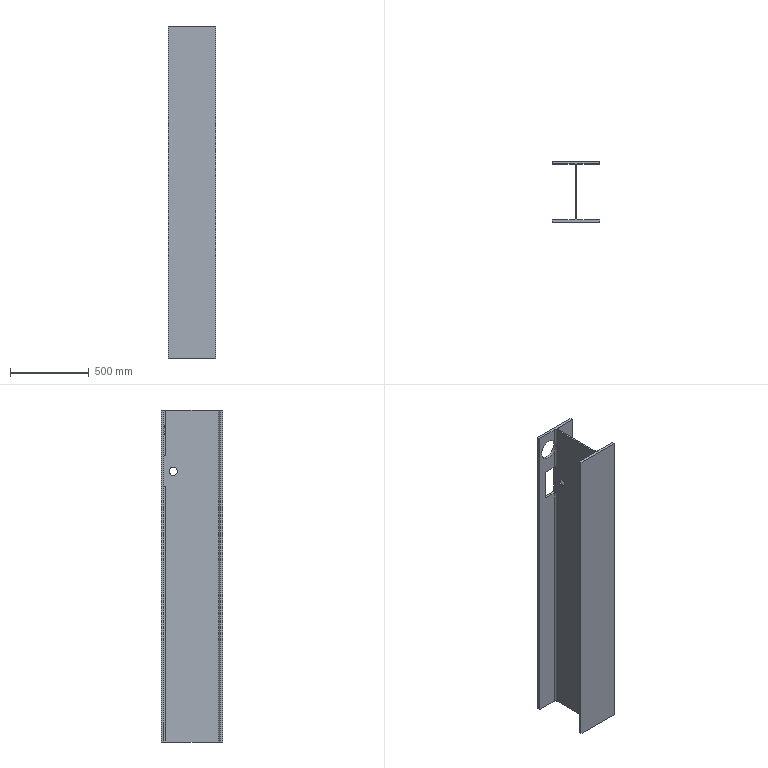Part | SolidWorks | features ICE 2, Extrusion 1 | 1 solid | 26 faces | box 300 x 390 x 2113 mm | volume 27642804 mm3 | plane 17 | cylinder 9 | commonest cylinder face diameters 26 x5 51 x2 125 x2
STEP:
#1=CARTESIAN_POINT('',(155.,289.5,1723.));
#2=VERTEX_POINT('',#1);
#3=CARTESIAN_POINT('',(155.,340.5,1723.));
#4=VERTEX_POINT('',#3);
#5=CARTESIAN_POINT('',(155.,315.,1723.));
#6=DIRECTION('',(1.,0.,0.));
#7=DIRECTION('',(0.,0.,1.));
#8=AXIS2_PLACEMENT_3D('',#5,#6,#7);
#9=CIRCLE('',#8,25.5);
#10=EDGE_CURVE('',#2,#4,#9,.T.);
#11=ORIENTED_EDGE('',*,*,#10,.T.);
#12=CARTESIAN_POINT('',(145.,340.5,1723.));
#13=VERTEX_POINT('',#12);
#14=CARTESIAN_POINT('',(300.001,340.5,1723.));
#15=DIRECTION('',(-1.,0.,0.));
#16=VECTOR('',#15,1000.);
#17=LINE('',#14,#16);
#18=EDGE_CURVE('',#4,#13,#17,.T.);
#19=ORIENTED_EDGE('',*,*,#18,.T.);
#20=CARTESIAN_POINT('',(145.,289.5,1723.));
#21=VERTEX_POINT('',#20);
#22=CARTESIAN_POINT('',(145.,315.,1723.));
#23=DIRECTION('',(-1.,0.,0.));
#24=DIRECTION('',(0.,-1.,0.));
#25=AXIS2_PLACEMENT_3D('',#22,#23,#24);
#26=CIRCLE('',#25,25.5);
#27=EDGE_CURVE('',#13,#21,#26,.T.);
#28=ORIENTED_EDGE('',*,*,#27,.T.);
#29=CARTESIAN_POINT('',(300.001,289.5,1723.));
#30=DIRECTION('',(-1.,0.,0.));
#31=VECTOR('',#30,1000.);
#32=LINE('',#29,#31);
#33=EDGE_CURVE('',#2,#21,#32,.T.);
#34=ORIENTED_EDGE('',*,*,#33,.F.);
#35=EDGE_LOOP('',(#11,#19,#28,#34));
#36=FACE_OUTER_BOUND('',#35,.T.);
#37=CARTESIAN_POINT('',(300.001,315.,1723.));
#38=DIRECTION('',(-1.,0.,0.));
#39=DIRECTION('',(0.,-1.,0.));
#40=AXIS2_PLACEMENT_3D('',#37,#38,#39);
#41=CYLINDRICAL_SURFACE('',#40,25.5);
#42=ADVANCED_FACE('',(#36),#41,.F.);
#43=CARTESIAN_POINT('',(82.,374.,2048.5));
#44=VERTEX_POINT('',#43);
#45=CARTESIAN_POINT('',(82.,374.,1923.5));
#46=VERTEX_POINT('',#45);
#47=CARTESIAN_POINT('',(82.,374.,1986.));
#48=DIRECTION('',(0.,-1.,0.));
#49=DIRECTION('',(-1.,0.,0.));
#50=AXIS2_PLACEMENT_3D('',#47,#48,#49);
#51=CIRCLE('',#50,62.5);
#52=EDGE_CURVE('',#44,#46,#51,.T.);
#53=ORIENTED_EDGE('',*,*,#52,.T.);
#54=CARTESIAN_POINT('',(82.,390.,1923.5));
#55=VERTEX_POINT('',#54);
#56=CARTESIAN_POINT('',(82.,-0.001,1923.5));
#57=DIRECTION('',(0.,1.,0.));
#58=VECTOR('',#57,1000.);
#59=LINE('',#56,#58);
#60=EDGE_CURVE('',#46,#55,#59,.T.);
#61=ORIENTED_EDGE('',*,*,#60,.T.);
#62=CARTESIAN_POINT('',(82.,390.,2048.5));
#63=VERTEX_POINT('',#62);
#64=CARTESIAN_POINT('',(82.,390.,1986.));
#65=DIRECTION('',(0.,1.,0.));
#66=DIRECTION('',(0.,0.,1.));
#67=AXIS2_PLACEMENT_3D('',#64,#65,#66);
#68=CIRCLE('',#67,62.5);
#69=EDGE_CURVE('',#55,#63,#68,.T.);
#70=ORIENTED_EDGE('',*,*,#69,.T.);
#71=CARTESIAN_POINT('',(82.,-0.001,2048.5));
#72=DIRECTION('',(0.,1.,0.));
#73=VECTOR('',#72,1000.);
#74=LINE('',#71,#73);
#75=EDGE_CURVE('',#44,#63,#74,.T.);
#76=ORIENTED_EDGE('',*,*,#75,.F.);
#77=EDGE_LOOP('',(#53,#61,#70,#76));
#78=FACE_OUTER_BOUND('',#77,.T.);
#79=CARTESIAN_POINT('',(82.,-0.001,1986.));
#80=DIRECTION('',(0.,1.,0.));
#81=DIRECTION('',(0.,0.,1.));
#82=AXIS2_PLACEMENT_3D('',#79,#80,#81);
#83=CYLINDRICAL_SURFACE('',#82,62.5);
#84=ADVANCED_FACE('',(#78),#83,.F.);
#85=CARTESIAN_POINT('',(132.,374.,1948.5));
#86=VERTEX_POINT('',#85);
#87=CARTESIAN_POINT('',(132.,374.,1823.));
#88=VERTEX_POINT('',#87);
#89=CARTESIAN_POINT('',(132.,374.,2113.));
#90=DIRECTION('',(0.,0.,-1.));
#91=VECTOR('',#90,1000.);
#92=LINE('',#89,#91);
#93=EDGE_CURVE('',#86,#88,#92,.T.);
#94=ORIENTED_EDGE('',*,*,#93,.T.);
#95=CARTESIAN_POINT('',(145.,361.,1823.));
#96=VERTEX_POINT('',#95);
#97=CARTESIAN_POINT('',(132.,361.,1823.));
#98=DIRECTION('',(0.,0.,1.));
#99=DIRECTION('',(1.,0.,0.));
#100=AXIS2_PLACEMENT_3D('',#97,#98,#99);
#101=CIRCLE('',#100,13.);
#102=EDGE_CURVE('',#96,#88,#101,.T.);
#103=ORIENTED_EDGE('',*,*,#102,.F.);
#104=CARTESIAN_POINT('',(145.,361.,2113.));
#105=VERTEX_POINT('',#104);
#106=CARTESIAN_POINT('',(145.,361.,2113.));
#107=DIRECTION('',(0.,0.,-1.));
#108=VECTOR('',#107,1000.);
#109=LINE('',#106,#108);
#110=EDGE_CURVE('',#105,#96,#109,.T.);
#111=ORIENTED_EDGE('',*,*,#110,.F.);
#112=CARTESIAN_POINT('',(132.,374.,2113.));
#113=VERTEX_POINT('',#112);
#114=CARTESIAN_POINT('',(132.,361.,2113.));
#115=DIRECTION('',(0.,0.,-1.));
#116=DIRECTION('',(-1.,0.,0.));
#117=AXIS2_PLACEMENT_3D('',#114,#115,#116);
#118=CIRCLE('',#117,13.);
#119=EDGE_CURVE('',#113,#105,#118,.T.);
#120=ORIENTED_EDGE('',*,*,#119,.F.);
#121=CARTESIAN_POINT('',(132.,374.,2023.5));
#122=VERTEX_POINT('',#121);
#123=CARTESIAN_POINT('',(132.,374.,2113.));
#124=DIRECTION('',(0.,0.,-1.));
#125=VECTOR('',#124,1000.);
#126=LINE('',#123,#125);
#127=EDGE_CURVE('',#113,#122,#126,.T.);
#128=ORIENTED_EDGE('',*,*,#127,.T.);
#129=CARTESIAN_POINT('',(132.,374.,1948.5));
#130=CARTESIAN_POINT('',(133.05,374.,1949.9));
#131=CARTESIAN_POINT('',(134.027,373.875,1951.324));
#132=CARTESIAN_POINT('',(135.848,373.452,1954.227));
#133=CARTESIAN_POINT('',(136.693,373.154,1955.705));
#134=CARTESIAN_POINT('',(137.866,372.609,1957.964));
#135=CARTESIAN_POINT('',(138.242,372.411,1958.726));
#136=CARTESIAN_POINT('',(138.957,371.99,1960.254));
#137=CARTESIAN_POINT('',(139.297,371.767,1961.019));
#138=CARTESIAN_POINT('',(140.264,371.067,1963.32));
#139=CARTESIAN_POINT('',(140.84,370.561,1964.862));
#140=CARTESIAN_POINT('',(141.865,369.499,1967.968));
#141=CARTESIAN_POINT('',(142.313,368.944,1969.532));
#142=CARTESIAN_POINT('',(143.089,367.82,1972.693));
#143=CARTESIAN_POINT('',(143.415,367.25,1974.289));
#144=CARTESIAN_POINT('',(143.813,366.435,1976.725));
#145=CARTESIAN_POINT('',(143.931,366.169,1977.545));
#146=CARTESIAN_POINT('',(144.134,365.673,1979.194));
#147=CARTESIAN_POINT('',(144.219,365.443,1980.023));
#148=CARTESIAN_POINT('',(144.357,365.043,1981.694));
#149=CARTESIAN_POINT('',(144.41,364.875,1982.537));
#150=CARTESIAN_POINT('',(144.481,364.638,1984.243));
#151=CARTESIAN_POINT('',(144.5,364.571,1985.107));
#152=CARTESIAN_POINT('',(144.5,364.57,1986.424));
#153=CARTESIAN_POINT('',(144.496,364.586,1986.863));
#154=CARTESIAN_POINT('',(144.478,364.649,1987.731));
#155=CARTESIAN_POINT('',(144.464,364.695,1988.161));
#156=CARTESIAN_POINT('',(144.411,364.871,1989.444));
#157=CARTESIAN_POINT('',(144.358,365.039,1990.288));
#158=CARTESIAN_POINT('',(144.221,365.438,1991.961));
#159=CARTESIAN_POINT('',(144.136,365.669,1992.79));
#160=CARTESIAN_POINT('',(143.933,366.164,1994.438));
#161=CARTESIAN_POINT('',(143.816,366.429,1995.259));
#162=CARTESIAN_POINT('',(143.418,367.245,1997.698));
#163=CARTESIAN_POINT('',(143.091,367.816,1999.298));
#164=CARTESIAN_POINT('',(142.314,368.943,2002.465));
#165=CARTESIAN_POINT('',(141.864,369.5,2004.033));
#166=CARTESIAN_POINT('',(140.836,370.564,2007.148));
#167=CARTESIAN_POINT('',(140.258,371.072,2008.695));
#168=CARTESIAN_POINT('',(139.286,371.774,2011.004));
#169=CARTESIAN_POINT('',(138.944,371.998,2011.775));
#170=CARTESIAN_POINT('',(138.228,372.418,2013.301));
#171=CARTESIAN_POINT('',(137.855,372.615,2014.057));
#172=CARTESIAN_POINT('',(136.686,373.156,2016.307));
#173=CARTESIAN_POINT('',(135.844,373.454,2017.78));
#174=CARTESIAN_POINT('',(134.026,373.875,2020.676));
#175=CARTESIAN_POINT('',(133.05,374.,2022.099));
#176=CARTESIAN_POINT('',(132.,374.,2023.5));
#177=B_SPLINE_CURVE_WITH_KNOTS('',3,(#129,#130,#131,#132,#133,#134,#135,#136,#137,#138,#139,#140,#141,#142,#143,#144,#145,#146,#147,#148,#149,#150,#151,#152,#153,#154,#155,#156,#157,#158,#159,#160,#161,#162,#163,#164,#165,#166,#167,#168,#169,#170,#171,#172,#173,#174,#175,#176),.UNSPECIFIED.,.F.,.F.,(4,2,2,2,2,2,2,2,2,2,2,2,2,2,2,2,2,2,2,2,2,2,2,4),(0.,0.005179,0.01036,0.01295,0.01554,0.02071,0.02589,0.03107,0.03366,0.03625,0.03884,0.04143,0.04272,0.04402,0.04661,0.0492,0.05179,0.05696,0.06214,0.06732,0.06991,0.0725,0.07768,0.08286),.UNSPECIFIED.);
#178=EDGE_CURVE('',#86,#122,#177,.T.);
#179=ORIENTED_EDGE('',*,*,#178,.F.);
#180=EDGE_LOOP('',(#94,#103,#111,#120,#128,#179));
#181=FACE_OUTER_BOUND('',#180,.T.);
#182=CARTESIAN_POINT('',(132.,361.,2113.));
#183=DIRECTION('',(0.,0.,-1.));
#184=DIRECTION('',(-1.,0.,0.));
#185=AXIS2_PLACEMENT_3D('',#182,#183,#184);
#186=CYLINDRICAL_SURFACE('',#185,13.);
#187=ADVANCED_FACE('',(#181),#186,.F.);
#188=CARTESIAN_POINT('',(0.,16.,0.));
#189=VERTEX_POINT('',#188);
#190=CARTESIAN_POINT('',(0.,0.,0.));
#191=VERTEX_POINT('',#190);
#192=CARTESIAN_POINT('',(0.,16.,0.));
#193=DIRECTION('',(0.,-1.,0.));
#194=VECTOR('',#193,1000.);
#195=LINE('',#192,#194);
#196=EDGE_CURVE('',#189,#191,#195,.T.);
#197=ORIENTED_EDGE('',*,*,#196,.T.);
#198=CARTESIAN_POINT('',(0.,0.,2113.));
#199=VERTEX_POINT('',#198);
#200=CARTESIAN_POINT('',(0.,0.,2113.));
#201=DIRECTION('',(0.,0.,-1.));
#202=VECTOR('',#201,1000.);
#203=LINE('',#200,#202);
#204=EDGE_CURVE('',#199,#191,#203,.T.);
#205=ORIENTED_EDGE('',*,*,#204,.F.);
#206=CARTESIAN_POINT('',(0.,16.,2113.));
#207=VERTEX_POINT('',#206);
#208=CARTESIAN_POINT('',(0.,16.,2113.));
#209=DIRECTION('',(0.,-1.,0.));
#210=VECTOR('',#209,1000.);
#211=LINE('',#208,#210);
#212=EDGE_CURVE('',#207,#199,#211,.T.);
#213=ORIENTED_EDGE('',*,*,#212,.F.);
#214=CARTESIAN_POINT('',(0.,16.,2113.));
#215=DIRECTION('',(0.,0.,-1.));
#216=VECTOR('',#215,1000.);
#217=LINE('',#214,#216);
#218=EDGE_CURVE('',#207,#189,#217,.T.);
#219=ORIENTED_EDGE('',*,*,#218,.T.);
#220=EDGE_LOOP('',(#197,#205,#213,#219));
#221=FACE_OUTER_BOUND('',#220,.T.);
#222=CARTESIAN_POINT('',(0.,16.,2113.));
#223=DIRECTION('',(1.,0.,0.));
#224=DIRECTION('',(0.,1.,0.));
#225=AXIS2_PLACEMENT_3D('',#222,#223,#224);
#226=PLANE('',#225);
#227=ADVANCED_FACE('',(#221),#226,.F.);
#228=CARTESIAN_POINT('',(300.,0.,0.));
#229=VERTEX_POINT('',#228);
#230=CARTESIAN_POINT('',(0.,0.,0.));
#231=DIRECTION('',(1.,0.,0.));
#232=VECTOR('',#231,1000.);
#233=LINE('',#230,#232);
#234=EDGE_CURVE('',#191,#229,#233,.T.);
#235=ORIENTED_EDGE('',*,*,#234,.T.);
#236=CARTESIAN_POINT('',(300.,0.,2113.));
#237=VERTEX_POINT('',#236);
#238=CARTESIAN_POINT('',(300.,0.,2113.));
#239=DIRECTION('',(0.,0.,-1.));
#240=VECTOR('',#239,1000.);
#241=LINE('',#238,#240);
#242=EDGE_CURVE('',#237,#229,#241,.T.);
#243=ORIENTED_EDGE('',*,*,#242,.F.);
#244=CARTESIAN_POINT('',(0.,0.,2113.));
#245=DIRECTION('',(1.,0.,0.));
#246=VECTOR('',#245,1000.);
#247=LINE('',#244,#246);
#248=EDGE_CURVE('',#199,#237,#247,.T.);
#249=ORIENTED_EDGE('',*,*,#248,.F.);
#250=ORIENTED_EDGE('',*,*,#204,.T.);
#251=EDGE_LOOP('',(#235,#243,#249,#250));
#252=FACE_OUTER_BOUND('',#251,.T.);
#253=CARTESIAN_POINT('',(0.,0.,2113.));
#254=DIRECTION('',(0.,1.,0.));
#255=DIRECTION('',(0.,0.,1.));
#256=AXIS2_PLACEMENT_3D('',#253,#254,#255);
#257=PLANE('',#256);
#258=ADVANCED_FACE('',(#252),#257,.F.);
#259=CARTESIAN_POINT('',(300.,16.,0.));
#260=VERTEX_POINT('',#259);
#261=CARTESIAN_POINT('',(300.,0.,0.));
#262=DIRECTION('',(0.,1.,0.));
#263=VECTOR('',#262,1000.);
#264=LINE('',#261,#263);
#265=EDGE_CURVE('',#229,#260,#264,.T.);
#266=ORIENTED_EDGE('',*,*,#265,.T.);
#267=CARTESIAN_POINT('',(300.,16.,2113.));
#268=VERTEX_POINT('',#267);
#269=CARTESIAN_POINT('',(300.,16.,2113.));
#270=DIRECTION('',(0.,0.,-1.));
#271=VECTOR('',#270,1000.);
#272=LINE('',#269,#271);
#273=EDGE_CURVE('',#268,#260,#272,.T.);
#274=ORIENTED_EDGE('',*,*,#273,.F.);
#275=CARTESIAN_POINT('',(300.,0.,2113.));
#276=DIRECTION('',(0.,1.,0.));
#277=VECTOR('',#276,1000.);
#278=LINE('',#275,#277);
#279=EDGE_CURVE('',#237,#268,#278,.T.);
#280=ORIENTED_EDGE('',*,*,#279,.F.);
#281=ORIENTED_EDGE('',*,*,#242,.T.);
#282=EDGE_LOOP('',(#266,#274,#280,#281));
#283=FACE_OUTER_BOUND('',#282,.T.);
#284=CARTESIAN_POINT('',(300.,0.,2113.));
#285=DIRECTION('',(-1.,0.,0.));
#286=DIRECTION('',(0.,0.,1.));
#287=AXIS2_PLACEMENT_3D('',#284,#285,#286);
#288=PLANE('',#287);
#289=ADVANCED_FACE('',(#283),#288,.F.);
#290=CARTESIAN_POINT('',(168.,16.,0.));
#291=VERTEX_POINT('',#290);
#292=CARTESIAN_POINT('',(300.,16.,0.));
#293=DIRECTION('',(-1.,0.,0.));
#294=VECTOR('',#293,1000.);
#295=LINE('',#292,#294);
#296=EDGE_CURVE('',#260,#291,#295,.T.);
#297=ORIENTED_EDGE('',*,*,#296,.T.);
#298=CARTESIAN_POINT('',(168.,16.,2113.));
#299=VERTEX_POINT('',#298);
#300=CARTESIAN_POINT('',(168.,16.,2113.));
#301=DIRECTION('',(0.,0.,-1.));
#302=VECTOR('',#301,1000.);
#303=LINE('',#300,#302);
#304=EDGE_CURVE('',#299,#291,#303,.T.);
#305=ORIENTED_EDGE('',*,*,#304,.F.);
#306=CARTESIAN_POINT('',(300.,16.,2113.));
#307=DIRECTION('',(-1.,0.,0.));
#308=VECTOR('',#307,1000.);
#309=LINE('',#306,#308);
#310=EDGE_CURVE('',#268,#299,#309,.T.);
#311=ORIENTED_EDGE('',*,*,#310,.F.);
#312=ORIENTED_EDGE('',*,*,#273,.T.);
#313=EDGE_LOOP('',(#297,#305,#311,#312));
#314=FACE_OUTER_BOUND('',#313,.T.);
#315=CARTESIAN_POINT('',(300.,16.,2113.));
#316=DIRECTION('',(0.,-1.,0.));
#317=DIRECTION('',(1.,0.,0.));
#318=AXIS2_PLACEMENT_3D('',#315,#316,#317);
#319=PLANE('',#318);
#320=ADVANCED_FACE('',(#314),#319,.F.);
#321=CARTESIAN_POINT('',(155.,29.,0.));
#322=VERTEX_POINT('',#321);
#323=CARTESIAN_POINT('',(168.,29.,0.));
#324=DIRECTION('',(0.,0.,-1.));
#325=DIRECTION('',(-1.,0.,0.));
#326=AXIS2_PLACEMENT_3D('',#323,#324,#325);
#327=CIRCLE('',#326,13.);
#328=EDGE_CURVE('',#291,#322,#327,.T.);
#329=ORIENTED_EDGE('',*,*,#328,.T.);
#330=CARTESIAN_POINT('',(155.,29.,2113.));
#331=VERTEX_POINT('',#330);
#332=CARTESIAN_POINT('',(155.,29.,2113.));
#333=DIRECTION('',(0.,0.,-1.));
#334=VECTOR('',#333,1000.);
#335=LINE('',#332,#334);
#336=EDGE_CURVE('',#331,#322,#335,.T.);
#337=ORIENTED_EDGE('',*,*,#336,.F.);
#338=CARTESIAN_POINT('',(168.,29.,2113.));
#339=DIRECTION('',(0.,0.,-1.));
#340=DIRECTION('',(-1.,0.,0.));
#341=AXIS2_PLACEMENT_3D('',#338,#339,#340);
#342=CIRCLE('',#341,13.);
#343=EDGE_CURVE('',#299,#331,#342,.T.);
#344=ORIENTED_EDGE('',*,*,#343,.F.);
#345=ORIENTED_EDGE('',*,*,#304,.T.);
#346=EDGE_LOOP('',(#329,#337,#344,#345));
#347=FACE_OUTER_BOUND('',#346,.T.);
#348=CARTESIAN_POINT('',(168.,29.,2113.));
#349=DIRECTION('',(0.,0.,-1.));
#350=DIRECTION('',(-1.,0.,0.));
#351=AXIS2_PLACEMENT_3D('',#348,#349,#350);
#352=CYLINDRICAL_SURFACE('',#351,13.);
#353=ADVANCED_FACE('',(#347),#352,.F.);
#354=ORIENTED_EDGE('',*,*,#10,.F.);
#355=CARTESIAN_POINT('',(155.,315.,1723.));
#356=DIRECTION('',(1.,0.,0.));
#357=DIRECTION('',(0.,0.,1.));
#358=AXIS2_PLACEMENT_3D('',#355,#356,#357);
#359=CIRCLE('',#358,25.5);
#360=EDGE_CURVE('',#4,#2,#359,.T.);
#361=ORIENTED_EDGE('',*,*,#360,.F.);
#362=EDGE_LOOP('',(#354,#361));
#363=FACE_BOUND('',#362,.T.);
#364=CARTESIAN_POINT('',(155.,361.,0.));
#365=VERTEX_POINT('',#364);
#366=CARTESIAN_POINT('',(155.,29.,0.));
#367=DIRECTION('',(0.,1.,0.));
#368=VECTOR('',#367,1000.);
#369=LINE('',#366,#368);
#370=EDGE_CURVE('',#322,#365,#369,.T.);
#371=ORIENTED_EDGE('',*,*,#370,.T.);
#372=CARTESIAN_POINT('',(155.,361.,2113.));
#373=VERTEX_POINT('',#372);
#374=CARTESIAN_POINT('',(155.,361.,2113.));
#375=DIRECTION('',(0.,0.,-1.));
#376=VECTOR('',#375,1000.);
#377=LINE('',#374,#376);
#378=EDGE_CURVE('',#373,#365,#377,.T.);
#379=ORIENTED_EDGE('',*,*,#378,.F.);
#380=CARTESIAN_POINT('',(155.,29.,2113.));
#381=DIRECTION('',(0.,1.,0.));
#382=VECTOR('',#381,1000.);
#383=LINE('',#380,#382);
#384=EDGE_CURVE('',#331,#373,#383,.T.);
#385=ORIENTED_EDGE('',*,*,#384,.F.);
#386=ORIENTED_EDGE('',*,*,#336,.T.);
#387=EDGE_LOOP('',(#371,#379,#385,#386));
#388=FACE_OUTER_BOUND('',#387,.T.);
#389=CARTESIAN_POINT('',(155.,29.,2113.));
#390=DIRECTION('',(-1.,0.,0.));
#391=DIRECTION('',(0.,0.,1.));
#392=AXIS2_PLACEMENT_3D('',#389,#390,#391);
#393=PLANE('',#392);
#394=ADVANCED_FACE('',(#363,#388),#393,.F.);
#395=CARTESIAN_POINT('',(168.,374.,0.));
#396=VERTEX_POINT('',#395);
#397=CARTESIAN_POINT('',(168.,361.,0.));
#398=DIRECTION('',(0.,0.,-1.));
#399=DIRECTION('',(-1.,0.,0.));
#400=AXIS2_PLACEMENT_3D('',#397,#398,#399);
#401=CIRCLE('',#400,13.);
#402=EDGE_CURVE('',#365,#396,#401,.T.);
#403=ORIENTED_EDGE('',*,*,#402,.T.);
#404=CARTESIAN_POINT('',(168.,374.,2113.));
#405=VERTEX_POINT('',#404);
#406=CARTESIAN_POINT('',(168.,374.,2113.));
#407=DIRECTION('',(0.,0.,-1.));
#408=VECTOR('',#407,1000.);
#409=LINE('',#406,#408);
#410=EDGE_CURVE('',#405,#396,#409,.T.);
#411=ORIENTED_EDGE('',*,*,#410,.F.);
#412=CARTESIAN_POINT('',(168.,361.,2113.));
#413=DIRECTION('',(0.,0.,-1.));
#414=DIRECTION('',(-1.,0.,0.));
#415=AXIS2_PLACEMENT_3D('',#412,#413,#414);
#416=CIRCLE('',#415,13.);
#417=EDGE_CURVE('',#373,#405,#416,.T.);
#418=ORIENTED_EDGE('',*,*,#417,.F.);
#419=ORIENTED_EDGE('',*,*,#378,.T.);
#420=EDGE_LOOP('',(#403,#411,#418,#419));
#421=FACE_OUTER_BOUND('',#420,.T.);
#422=CARTESIAN_POINT('',(168.,361.,2113.));
#423=DIRECTION('',(0.,0.,-1.));
#424=DIRECTION('',(-1.,0.,0.));
#425=AXIS2_PLACEMENT_3D('',#422,#423,#424);
#426=CYLINDRICAL_SURFACE('',#425,13.);
#427=ADVANCED_FACE('',(#421),#426,.F.);
#428=CARTESIAN_POINT('',(300.,374.,0.));
#429=VERTEX_POINT('',#428);
#430=CARTESIAN_POINT('',(168.,374.,0.));
#431=DIRECTION('',(1.,0.,0.));
#432=VECTOR('',#431,1000.);
#433=LINE('',#430,#432);
#434=EDGE_CURVE('',#396,#429,#433,.T.);
#435=ORIENTED_EDGE('',*,*,#434,.T.);
#436=CARTESIAN_POINT('',(300.,374.,2113.));
#437=VERTEX_POINT('',#436);
#438=CARTESIAN_POINT('',(300.,374.,2113.));
#439=DIRECTION('',(0.,0.,-1.));
#440=VECTOR('',#439,1000.);
#441=LINE('',#438,#440);
#442=EDGE_CURVE('',#437,#429,#441,.T.);
#443=ORIENTED_EDGE('',*,*,#442,.F.);
#444=CARTESIAN_POINT('',(168.,374.,2113.));
#445=DIRECTION('',(1.,0.,0.));
#446=VECTOR('',#445,1000.);
#447=LINE('',#444,#446);
#448=EDGE_CURVE('',#405,#437,#447,.T.);
#449=ORIENTED_EDGE('',*,*,#448,.F.);
#450=ORIENTED_EDGE('',*,*,#410,.T.);
#451=EDGE_LOOP('',(#435,#443,#449,#450));
#452=FACE_OUTER_BOUND('',#451,.T.);
#453=CARTESIAN_POINT('',(168.,374.,2113.));
#454=DIRECTION('',(0.,1.,0.));
#455=DIRECTION('',(0.,0.,1.));
#456=AXIS2_PLACEMENT_3D('',#453,#454,#455);
#457=PLANE('',#456);
#458=ADVANCED_FACE('',(#452),#457,.F.);
#459=CARTESIAN_POINT('',(300.,390.,0.));
#460=VERTEX_POINT('',#459);
#461=CARTESIAN_POINT('',(300.,374.,0.));
#462=DIRECTION('',(0.,1.,0.));
#463=VECTOR('',#462,1000.);
#464=LINE('',#461,#463);
#465=EDGE_CURVE('',#429,#460,#464,.T.);
#466=ORIENTED_EDGE('',*,*,#465,.T.);
#467=CARTESIAN_POINT('',(300.,390.,2113.));
#468=VERTEX_POINT('',#467);
#469=CARTESIAN_POINT('',(300.,390.,2113.));
#470=DIRECTION('',(0.,0.,-1.));
#471=VECTOR('',#470,1000.);
#472=LINE('',#469,#471);
#473=EDGE_CURVE('',#468,#460,#472,.T.);
#474=ORIENTED_EDGE('',*,*,#473,.F.);
#475=CARTESIAN_POINT('',(300.,374.,2113.));
#476=DIRECTION('',(0.,1.,0.));
#477=VECTOR('',#476,1000.);
#478=LINE('',#475,#477);
#479=EDGE_CURVE('',#437,#468,#478,.T.);
#480=ORIENTED_EDGE('',*,*,#479,.F.);
#481=ORIENTED_EDGE('',*,*,#442,.T.);
#482=EDGE_LOOP('',(#466,#474,#480,#481));
#483=FACE_OUTER_BOUND('',#482,.T.);
#484=CARTESIAN_POINT('',(300.,374.,2113.));
#485=DIRECTION('',(-1.,0.,0.));
#486=DIRECTION('',(0.,-1.,0.));
#487=AXIS2_PLACEMENT_3D('',#484,#485,#486);
#488=PLANE('',#487);
#489=ADVANCED_FACE('',(#483),#488,.F.);
#490=CARTESIAN_POINT('',(145.,390.,1823.));
#491=VERTEX_POINT('',#490);
#492=CARTESIAN_POINT('',(145.,390.,1623.));
#493=VERTEX_POINT('',#492);
#494=CARTESIAN_POINT('',(145.,390.,1623.));
#495=DIRECTION('',(0.,0.,-1.));
#496=VECTOR('',#495,1000.);
#497=LINE('',#494,#496);
#498=EDGE_CURVE('',#491,#493,#497,.T.);
#499=ORIENTED_EDGE('',*,*,#498,.F.);
#500=CARTESIAN_POINT('',(55.,390.,1823.));
#501=VERTEX_POINT('',#500);
#502=CARTESIAN_POINT('',(145.,390.,1823.));
#503=DIRECTION('',(1.,0.,0.));
#504=VECTOR('',#503,1000.);
#505=LINE('',#502,#504);
#506=EDGE_CURVE('',#501,#491,#505,.T.);
#507=ORIENTED_EDGE('',*,*,#506,.F.);
#508=CARTESIAN_POINT('',(55.,390.,1623.));
#509=VERTEX_POINT('',#508);
#510=CARTESIAN_POINT('',(55.,390.,1623.));
#511=DIRECTION('',(0.,0.,1.));
#512=VECTOR('',#511,1000.);
#513=LINE('',#510,#512);
#514=EDGE_CURVE('',#509,#501,#513,.T.);
#515=ORIENTED_EDGE('',*,*,#514,.F.);
#516=CARTESIAN_POINT('',(145.,390.,1623.));
#517=DIRECTION('',(-1.,0.,0.));
#518=VECTOR('',#517,1000.);
#519=LINE('',#516,#518);
#520=EDGE_CURVE('',#493,#509,#519,.T.);
#521=ORIENTED_EDGE('',*,*,#520,.F.);
#522=EDGE_LOOP('',(#499,#507,#515,#521));
#523=FACE_BOUND('',#522,.T.);
#524=CARTESIAN_POINT('',(82.,390.,1986.));
#525=DIRECTION('',(0.,1.,0.));
#526=DIRECTION('',(0.,0.,1.));
#527=AXIS2_PLACEMENT_3D('',#524,#525,#526);
#528=CIRCLE('',#527,62.5);
#529=EDGE_CURVE('',#63,#55,#528,.T.);
#530=ORIENTED_EDGE('',*,*,#529,.F.);
#531=ORIENTED_EDGE('',*,*,#69,.F.);
#532=EDGE_LOOP('',(#530,#531));
#533=FACE_BOUND('',#532,.T.);
#534=CARTESIAN_POINT('',(0.,390.,0.));
#535=VERTEX_POINT('',#534);
#536=CARTESIAN_POINT('',(300.,390.,0.));
#537=DIRECTION('',(-1.,0.,0.));
#538=VECTOR('',#537,1000.);
#539=LINE('',#536,#538);
#540=EDGE_CURVE('',#460,#535,#539,.T.);
#541=ORIENTED_EDGE('',*,*,#540,.T.);
#542=CARTESIAN_POINT('',(0.,390.,2113.));
#543=VERTEX_POINT('',#542);
#544=CARTESIAN_POINT('',(0.,390.,2113.));
#545=DIRECTION('',(0.,0.,-1.));
#546=VECTOR('',#545,1000.);
#547=LINE('',#544,#546);
#548=EDGE_CURVE('',#543,#535,#547,.T.);
#549=ORIENTED_EDGE('',*,*,#548,.F.);
#550=CARTESIAN_POINT('',(300.,390.,2113.));
#551=DIRECTION('',(-1.,0.,0.));
#552=VECTOR('',#551,1000.);
#553=LINE('',#550,#552);
#554=EDGE_CURVE('',#468,#543,#553,.T.);
#555=ORIENTED_EDGE('',*,*,#554,.F.);
#556=ORIENTED_EDGE('',*,*,#473,.T.);
#557=EDGE_LOOP('',(#541,#549,#555,#556));
#558=FACE_OUTER_BOUND('',#557,.T.);
#559=CARTESIAN_POINT('',(300.,390.,2113.));
#560=DIRECTION('',(0.,-1.,0.));
#561=DIRECTION('',(0.,0.,-1.));
#562=AXIS2_PLACEMENT_3D('',#559,#560,#561);
#563=PLANE('',#562);
#564=ADVANCED_FACE('',(#523,#533,#558),#563,.F.);
#565=CARTESIAN_POINT('',(0.,374.,0.));
#566=VERTEX_POINT('',#565);
#567=CARTESIAN_POINT('',(0.,390.,0.));
#568=DIRECTION('',(0.,-1.,0.));
#569=VECTOR('',#568,1000.);
#570=LINE('',#567,#569);
#571=EDGE_CURVE('',#535,#566,#570,.T.);
#572=ORIENTED_EDGE('',*,*,#571,.T.);
#573=CARTESIAN_POINT('',(0.,374.,2113.));
#574=VERTEX_POINT('',#573);
#575=CARTESIAN_POINT('',(0.,374.,2113.));
#576=DIRECTION('',(0.,0.,-1.));
#577=VECTOR('',#576,1000.);
#578=LINE('',#575,#577);
#579=EDGE_CURVE('',#574,#566,#578,.T.);
#580=ORIENTED_EDGE('',*,*,#579,.F.);
#581=CARTESIAN_POINT('',(0.,390.,2113.));
#582=DIRECTION('',(0.,-1.,0.));
#583=VECTOR('',#582,1000.);
#584=LINE('',#581,#583);
#585=EDGE_CURVE('',#543,#574,#584,.T.);
#586=ORIENTED_EDGE('',*,*,#585,.F.);
#587=ORIENTED_EDGE('',*,*,#548,.T.);
#588=EDGE_LOOP('',(#572,#580,#586,#587));
#589=FACE_OUTER_BOUND('',#588,.T.);
#590=CARTESIAN_POINT('',(0.,390.,2113.));
#591=DIRECTION('',(1.,0.,0.));
#592=DIRECTION('',(0.,0.,-1.));
#593=AXIS2_PLACEMENT_3D('',#590,#591,#592);
#594=PLANE('',#593);
#595=ADVANCED_FACE('',(#589),#594,.F.);
#596=CARTESIAN_POINT('',(55.,374.,1823.));
#597=VERTEX_POINT('',#596);
#598=CARTESIAN_POINT('',(55.,374.,1623.));
#599=VERTEX_POINT('',#598);
#600=CARTESIAN_POINT('',(55.,374.,1623.));
#601=DIRECTION('',(0.,0.,-1.));
#602=VECTOR('',#601,1000.);
#603=LINE('',#600,#602);
#604=EDGE_CURVE('',#597,#599,#603,.T.);
#605=ORIENTED_EDGE('',*,*,#604,.F.);
#606=CARTESIAN_POINT('',(145.,374.,1823.));
#607=DIRECTION('',(-1.,0.,0.));
#608=VECTOR('',#607,1000.);
#609=LINE('',#606,#608);
#610=EDGE_CURVE('',#88,#597,#609,.T.);
#611=ORIENTED_EDGE('',*,*,#610,.F.);
#612=ORIENTED_EDGE('',*,*,#93,.F.);
#613=CARTESIAN_POINT('',(82.,374.,1986.));
#614=DIRECTION('',(0.,-1.,0.));
#615=DIRECTION('',(-1.,0.,0.));
#616=AXIS2_PLACEMENT_3D('',#613,#614,#615);
#617=CIRCLE('',#616,62.5);
#618=EDGE_CURVE('',#46,#86,#617,.T.);
#619=ORIENTED_EDGE('',*,*,#618,.F.);
#620=ORIENTED_EDGE('',*,*,#52,.F.);
#621=CARTESIAN_POINT('',(82.,374.,1986.));
#622=DIRECTION('',(0.,-1.,0.));
#623=DIRECTION('',(-1.,0.,0.));
#624=AXIS2_PLACEMENT_3D('',#621,#622,#623);
#625=CIRCLE('',#624,62.5);
#626=EDGE_CURVE('',#122,#44,#625,.T.);
#627=ORIENTED_EDGE('',*,*,#626,.F.);
#628=ORIENTED_EDGE('',*,*,#127,.F.);
#629=CARTESIAN_POINT('',(0.,374.,2113.));
#630=DIRECTION('',(1.,0.,0.));
#631=VECTOR('',#630,1000.);
#632=LINE('',#629,#631);
#633=EDGE_CURVE('',#574,#113,#632,.T.);
#634=ORIENTED_EDGE('',*,*,#633,.F.);
#635=ORIENTED_EDGE('',*,*,#579,.T.);
#636=CARTESIAN_POINT('',(132.,374.,0.));
#637=VERTEX_POINT('',#636);
#638=CARTESIAN_POINT('',(0.,374.,0.));
#639=DIRECTION('',(1.,0.,0.));
#640=VECTOR('',#639,1000.);
#641=LINE('',#638,#640);
#642=EDGE_CURVE('',#566,#637,#641,.T.);
#643=ORIENTED_EDGE('',*,*,#642,.T.);
#644=CARTESIAN_POINT('',(132.,374.,1623.));
#645=VERTEX_POINT('',#644);
#646=CARTESIAN_POINT('',(132.,374.,2113.));
#647=DIRECTION('',(0.,0.,-1.));
#648=VECTOR('',#647,1000.);
#649=LINE('',#646,#648);
#650=EDGE_CURVE('',#645,#637,#649,.T.);
#651=ORIENTED_EDGE('',*,*,#650,.F.);
#652=CARTESIAN_POINT('',(145.,374.,1623.));
#653=DIRECTION('',(1.,0.,0.));
#654=VECTOR('',#653,1000.);
#655=LINE('',#652,#654);
#656=EDGE_CURVE('',#599,#645,#655,.T.);
#657=ORIENTED_EDGE('',*,*,#656,.F.);
#658=EDGE_LOOP('',(#605,#611,#612,#619,#620,#627,#628,#634,#635,#643,#651,#657));
#659=FACE_OUTER_BOUND('',#658,.T.);
#660=CARTESIAN_POINT('',(0.,374.,2113.));
#661=DIRECTION('',(0.,1.,0.));
#662=DIRECTION('',(-1.,0.,0.));
#663=AXIS2_PLACEMENT_3D('',#660,#661,#662);
#664=PLANE('',#663);
#665=ADVANCED_FACE('',(#659),#664,.F.);
#666=CARTESIAN_POINT('',(145.,361.,1623.));
#667=VERTEX_POINT('',#666);
#668=CARTESIAN_POINT('',(145.,361.,0.));
#669=VERTEX_POINT('',#668);
#670=CARTESIAN_POINT('',(145.,361.,2113.));
#671=DIRECTION('',(0.,0.,-1.));
#672=VECTOR('',#671,1000.);
#673=LINE('',#670,#672);
#674=EDGE_CURVE('',#667,#669,#673,.T.);
#675=ORIENTED_EDGE('',*,*,#674,.F.);
#676=CARTESIAN_POINT('',(132.,361.,1623.));
#677=DIRECTION('',(0.,0.,-1.));
#678=DIRECTION('',(-1.,0.,0.));
#679=AXIS2_PLACEMENT_3D('',#676,#677,#678);
#680=CIRCLE('',#679,13.);
#681=EDGE_CURVE('',#645,#667,#680,.T.);
#682=ORIENTED_EDGE('',*,*,#681,.F.);
#683=ORIENTED_EDGE('',*,*,#650,.T.);
#684=CARTESIAN_POINT('',(132.,361.,0.));
#685=DIRECTION('',(0.,0.,-1.));
#686=DIRECTION('',(-1.,0.,0.));
#687=AXIS2_PLACEMENT_3D('',#684,#685,#686);
#688=CIRCLE('',#687,13.);
#689=EDGE_CURVE('',#637,#669,#688,.T.);
#690=ORIENTED_EDGE('',*,*,#689,.T.);
#691=EDGE_LOOP('',(#675,#682,#683,#690));
#692=FACE_OUTER_BOUND('',#691,.T.);
#693=CARTESIAN_POINT('',(132.,361.,2113.));
#694=DIRECTION('',(0.,0.,-1.));
#695=DIRECTION('',(-1.,0.,0.));
#696=AXIS2_PLACEMENT_3D('',#693,#694,#695);
#697=CYLINDRICAL_SURFACE('',#696,13.);
#698=ADVANCED_FACE('',(#692),#697,.F.);
#699=CARTESIAN_POINT('',(145.,315.,1723.));
#700=DIRECTION('',(-1.,0.,0.));
#701=DIRECTION('',(0.,-1.,0.));
#702=AXIS2_PLACEMENT_3D('',#699,#700,#701);
#703=CIRCLE('',#702,25.5);
#704=EDGE_CURVE('',#21,#13,#703,.T.);
#705=ORIENTED_EDGE('',*,*,#704,.F.);
#706=ORIENTED_EDGE('',*,*,#27,.F.);
#707=EDGE_LOOP('',(#705,#706));
#708=FACE_BOUND('',#707,.T.);
#709=CARTESIAN_POINT('',(145.,29.,0.));
#710=VERTEX_POINT('',#709);
#711=CARTESIAN_POINT('',(145.,361.,0.));
#712=DIRECTION('',(0.,-1.,0.));
#713=VECTOR('',#712,1000.);
#714=LINE('',#711,#713);
#715=EDGE_CURVE('',#669,#710,#714,.T.);
#716=ORIENTED_EDGE('',*,*,#715,.T.);
#717=CARTESIAN_POINT('',(145.,29.,2113.));
#718=VERTEX_POINT('',#717);
#719=CARTESIAN_POINT('',(145.,29.,2113.));
#720=DIRECTION('',(0.,0.,-1.));
#721=VECTOR('',#720,1000.);
#722=LINE('',#719,#721);
#723=EDGE_CURVE('',#718,#710,#722,.T.);
#724=ORIENTED_EDGE('',*,*,#723,.F.);
#725=CARTESIAN_POINT('',(145.,361.,2113.));
#726=DIRECTION('',(0.,-1.,0.));
#727=VECTOR('',#726,1000.);
#728=LINE('',#725,#727);
#729=EDGE_CURVE('',#105,#718,#728,.T.);
#730=ORIENTED_EDGE('',*,*,#729,.F.);
#731=ORIENTED_EDGE('',*,*,#110,.T.);
#732=CARTESIAN_POINT('',(145.,-0.001,1823.));
#733=DIRECTION('',(0.,1.,0.));
#734=VECTOR('',#733,1000.);
#735=LINE('',#732,#734);
#736=EDGE_CURVE('',#96,#491,#735,.T.);
#737=ORIENTED_EDGE('',*,*,#736,.T.);
#738=ORIENTED_EDGE('',*,*,#498,.T.);
#739=CARTESIAN_POINT('',(145.,-0.001,1623.));
#740=DIRECTION('',(0.,1.,0.));
#741=VECTOR('',#740,1000.);
#742=LINE('',#739,#741);
#743=EDGE_CURVE('',#667,#493,#742,.T.);
#744=ORIENTED_EDGE('',*,*,#743,.F.);
#745=ORIENTED_EDGE('',*,*,#674,.T.);
#746=EDGE_LOOP('',(#716,#724,#730,#731,#737,#738,#744,#745));
#747=FACE_OUTER_BOUND('',#746,.T.);
#748=CARTESIAN_POINT('',(145.,361.,2113.));
#749=DIRECTION('',(1.,0.,0.));
#750=DIRECTION('',(0.,1.,0.));
#751=AXIS2_PLACEMENT_3D('',#748,#749,#750);
#752=PLANE('',#751);
#753=ADVANCED_FACE('',(#708,#747),#752,.F.);
#754=CARTESIAN_POINT('',(132.,16.,0.));
#755=VERTEX_POINT('',#754);
#756=CARTESIAN_POINT('',(132.,29.,0.));
#757=DIRECTION('',(0.,0.,-1.));
#758=DIRECTION('',(-1.,0.,0.));
#759=AXIS2_PLACEMENT_3D('',#756,#757,#758);
#760=CIRCLE('',#759,13.);
#761=EDGE_CURVE('',#710,#755,#760,.T.);
#762=ORIENTED_EDGE('',*,*,#761,.T.);
#763=CARTESIAN_POINT('',(132.,16.,2113.));
#764=VERTEX_POINT('',#763);
#765=CARTESIAN_POINT('',(132.,16.,2113.));
#766=DIRECTION('',(0.,0.,-1.));
#767=VECTOR('',#766,1000.);
#768=LINE('',#765,#767);
#769=EDGE_CURVE('',#764,#755,#768,.T.);
#770=ORIENTED_EDGE('',*,*,#769,.F.);
#771=CARTESIAN_POINT('',(132.,29.,2113.));
#772=DIRECTION('',(0.,0.,-1.));
#773=DIRECTION('',(-1.,0.,0.));
#774=AXIS2_PLACEMENT_3D('',#771,#772,#773);
#775=CIRCLE('',#774,13.);
#776=EDGE_CURVE('',#718,#764,#775,.T.);
#777=ORIENTED_EDGE('',*,*,#776,.F.);
#778=ORIENTED_EDGE('',*,*,#723,.T.);
#779=EDGE_LOOP('',(#762,#770,#777,#778));
#780=FACE_OUTER_BOUND('',#779,.T.);
#781=CARTESIAN_POINT('',(132.,29.,2113.));
#782=DIRECTION('',(0.,0.,-1.));
#783=DIRECTION('',(-1.,0.,0.));
#784=AXIS2_PLACEMENT_3D('',#781,#782,#783);
#785=CYLINDRICAL_SURFACE('',#784,13.);
#786=ADVANCED_FACE('',(#780),#785,.F.);
#787=CARTESIAN_POINT('',(132.,16.,0.));
#788=DIRECTION('',(-1.,0.,0.));
#789=VECTOR('',#788,1000.);
#790=LINE('',#787,#789);
#791=EDGE_CURVE('',#755,#189,#790,.T.);
#792=ORIENTED_EDGE('',*,*,#791,.T.);
#793=ORIENTED_EDGE('',*,*,#218,.F.);
#794=CARTESIAN_POINT('',(132.,16.,2113.));
#795=DIRECTION('',(-1.,0.,0.));
#796=VECTOR('',#795,1000.);
#797=LINE('',#794,#796);
#798=EDGE_CURVE('',#764,#207,#797,.T.);
#799=ORIENTED_EDGE('',*,*,#798,.F.);
#800=ORIENTED_EDGE('',*,*,#769,.T.);
#801=EDGE_LOOP('',(#792,#793,#799,#800));
#802=FACE_OUTER_BOUND('',#801,.T.);
#803=CARTESIAN_POINT('',(132.,16.,2113.));
#804=DIRECTION('',(0.,-1.,0.));
#805=DIRECTION('',(1.,0.,0.));
#806=AXIS2_PLACEMENT_3D('',#803,#804,#805);
#807=PLANE('',#806);
#808=ADVANCED_FACE('',(#802),#807,.F.);
#809=ORIENTED_EDGE('',*,*,#212,.T.);
#810=ORIENTED_EDGE('',*,*,#248,.T.);
#811=ORIENTED_EDGE('',*,*,#279,.T.);
#812=ORIENTED_EDGE('',*,*,#310,.T.);
#813=ORIENTED_EDGE('',*,*,#343,.T.);
#814=ORIENTED_EDGE('',*,*,#384,.T.);
#815=ORIENTED_EDGE('',*,*,#417,.T.);
#816=ORIENTED_EDGE('',*,*,#448,.T.);
#817=ORIENTED_EDGE('',*,*,#479,.T.);
#818=ORIENTED_EDGE('',*,*,#554,.T.);
#819=ORIENTED_EDGE('',*,*,#585,.T.);
#820=ORIENTED_EDGE('',*,*,#633,.T.);
#821=ORIENTED_EDGE('',*,*,#119,.T.);
#822=ORIENTED_EDGE('',*,*,#729,.T.);
#823=ORIENTED_EDGE('',*,*,#776,.T.);
#824=ORIENTED_EDGE('',*,*,#798,.T.);
#825=EDGE_LOOP('',(#809,#810,#811,#812,#813,#814,#815,#816,#817,#818,#819,#820,#821,#822,#823,#824));
#826=FACE_OUTER_BOUND('',#825,.T.);
#827=CARTESIAN_POINT('',(168.,29.,2113.));
#828=DIRECTION('',(0.,0.,-1.));
#829=DIRECTION('',(-1.,0.,0.));
#830=AXIS2_PLACEMENT_3D('',#827,#828,#829);
#831=PLANE('',#830);
#832=ADVANCED_FACE('',(#826),#831,.F.);
#833=ORIENTED_EDGE('',*,*,#196,.F.);
#834=ORIENTED_EDGE('',*,*,#791,.F.);
#835=ORIENTED_EDGE('',*,*,#761,.F.);
#836=ORIENTED_EDGE('',*,*,#715,.F.);
#837=ORIENTED_EDGE('',*,*,#689,.F.);
#838=ORIENTED_EDGE('',*,*,#642,.F.);
#839=ORIENTED_EDGE('',*,*,#571,.F.);
#840=ORIENTED_EDGE('',*,*,#540,.F.);
#841=ORIENTED_EDGE('',*,*,#465,.F.);
#842=ORIENTED_EDGE('',*,*,#434,.F.);
#843=ORIENTED_EDGE('',*,*,#402,.F.);
#844=ORIENTED_EDGE('',*,*,#370,.F.);
#845=ORIENTED_EDGE('',*,*,#328,.F.);
#846=ORIENTED_EDGE('',*,*,#296,.F.);
#847=ORIENTED_EDGE('',*,*,#265,.F.);
#848=ORIENTED_EDGE('',*,*,#234,.F.);
#849=EDGE_LOOP('',(#833,#834,#835,#836,#837,#838,#839,#840,#841,#842,#843,#844,#845,#846,#847,#848));
#850=FACE_OUTER_BOUND('',#849,.T.);
#851=CARTESIAN_POINT('',(168.,29.,0.));
#852=DIRECTION('',(0.,0.,-1.));
#853=DIRECTION('',(-1.,0.,0.));
#854=AXIS2_PLACEMENT_3D('',#851,#852,#853);
#855=PLANE('',#854);
#856=ADVANCED_FACE('',(#850),#855,.T.);
#857=ORIENTED_EDGE('',*,*,#610,.T.);
#858=CARTESIAN_POINT('',(55.,-0.001,1823.));
#859=DIRECTION('',(0.,1.,0.));
#860=VECTOR('',#859,1000.);
#861=LINE('',#858,#860);
#862=EDGE_CURVE('',#597,#501,#861,.T.);
#863=ORIENTED_EDGE('',*,*,#862,.T.);
#864=ORIENTED_EDGE('',*,*,#506,.T.);
#865=ORIENTED_EDGE('',*,*,#736,.F.);
#866=ORIENTED_EDGE('',*,*,#102,.T.);
#867=EDGE_LOOP('',(#857,#863,#864,#865,#866));
#868=FACE_OUTER_BOUND('',#867,.T.);
#869=CARTESIAN_POINT('',(145.,-0.001,1823.));
#870=DIRECTION('',(0.,0.,1.));
#871=DIRECTION('',(1.,0.,0.));
#872=AXIS2_PLACEMENT_3D('',#869,#870,#871);
#873=PLANE('',#872);
#874=ADVANCED_FACE('',(#868),#873,.F.);
#875=ORIENTED_EDGE('',*,*,#604,.T.);
#876=CARTESIAN_POINT('',(55.,-0.001,1623.));
#877=DIRECTION('',(0.,1.,0.));
#878=VECTOR('',#877,1000.);
#879=LINE('',#876,#878);
#880=EDGE_CURVE('',#599,#509,#879,.T.);
#881=ORIENTED_EDGE('',*,*,#880,.T.);
#882=ORIENTED_EDGE('',*,*,#514,.T.);
#883=ORIENTED_EDGE('',*,*,#862,.F.);
#884=EDGE_LOOP('',(#875,#881,#882,#883));
#885=FACE_OUTER_BOUND('',#884,.T.);
#886=CARTESIAN_POINT('',(55.,-0.001,1623.));
#887=DIRECTION('',(-1.,0.,0.));
#888=DIRECTION('',(0.,0.,1.));
#889=AXIS2_PLACEMENT_3D('',#886,#887,#888);
#890=PLANE('',#889);
#891=ADVANCED_FACE('',(#885),#890,.F.);
#892=ORIENTED_EDGE('',*,*,#656,.T.);
#893=ORIENTED_EDGE('',*,*,#681,.T.);
#894=ORIENTED_EDGE('',*,*,#743,.T.);
#895=ORIENTED_EDGE('',*,*,#520,.T.);
#896=ORIENTED_EDGE('',*,*,#880,.F.);
#897=EDGE_LOOP('',(#892,#893,#894,#895,#896));
#898=FACE_OUTER_BOUND('',#897,.T.);
#899=CARTESIAN_POINT('',(145.,-0.001,1623.));
#900=DIRECTION('',(0.,0.,-1.));
#901=DIRECTION('',(-1.,0.,0.));
#902=AXIS2_PLACEMENT_3D('',#899,#900,#901);
#903=PLANE('',#902);
#904=ADVANCED_FACE('',(#898),#903,.F.);
#905=ORIENTED_EDGE('',*,*,#60,.F.);
#906=ORIENTED_EDGE('',*,*,#618,.T.);
#907=ORIENTED_EDGE('',*,*,#178,.T.);
#908=ORIENTED_EDGE('',*,*,#626,.T.);
#909=ORIENTED_EDGE('',*,*,#75,.T.);
#910=ORIENTED_EDGE('',*,*,#529,.T.);
#911=EDGE_LOOP('',(#905,#906,#907,#908,#909,#910));
#912=FACE_OUTER_BOUND('',#911,.T.);
#913=CARTESIAN_POINT('',(82.,-0.001,1986.));
#914=DIRECTION('',(0.,1.,0.));
#915=DIRECTION('',(0.,0.,1.));
#916=AXIS2_PLACEMENT_3D('',#913,#914,#915);
#917=CYLINDRICAL_SURFACE('',#916,62.5);
#918=ADVANCED_FACE('',(#912),#917,.F.);
#919=ORIENTED_EDGE('',*,*,#18,.F.);
#920=ORIENTED_EDGE('',*,*,#360,.T.);
#921=ORIENTED_EDGE('',*,*,#33,.T.);
#922=ORIENTED_EDGE('',*,*,#704,.T.);
#923=EDGE_LOOP('',(#919,#920,#921,#922));
#924=FACE_OUTER_BOUND('',#923,.T.);
#925=CARTESIAN_POINT('',(300.001,315.,1723.));
#926=DIRECTION('',(-1.,0.,0.));
#927=DIRECTION('',(0.,-1.,0.));
#928=AXIS2_PLACEMENT_3D('',#925,#926,#927);
#929=CYLINDRICAL_SURFACE('',#928,25.5);
#930=ADVANCED_FACE('',(#924),#929,.F.);
#931=CLOSED_SHELL('',(#42,#84,#187,#227,#258,#289,#320,#353,#394,#427,#458,#489,#564,#595,#665,#698,#753,#786,#808,#832,#856,#874,#891,#904,#918,#930));
#932=MANIFOLD_SOLID_BREP('',#931);
#933=CARTESIAN_POINT('',(0.,0.,0.));
#934=DIRECTION('',(0.,0.,1.));
#935=DIRECTION('',(1.,0.,0.));
#936=AXIS2_PLACEMENT_3D('',#933,#934,#935);
#937=(LENGTH_UNIT()NAMED_UNIT(*)SI_UNIT(.MILLI.,.METRE.));
#938=UNCERTAINTY_MEASURE_WITH_UNIT(LENGTH_MEASURE(0.00001),#937,'','');
#939=(NAMED_UNIT(*)PLANE_ANGLE_UNIT()SI_UNIT($,.RADIAN.));
#940=(NAMED_UNIT(*)SI_UNIT($,.STERADIAN.)SOLID_ANGLE_UNIT());
#941=(GEOMETRIC_REPRESENTATION_CONTEXT(3)GLOBAL_UNCERTAINTY_ASSIGNED_CONTEXT((#938))GLOBAL_UNIT_ASSIGNED_CONTEXT((#937,#939,#940))REPRESENTATION_CONTEXT('',''));
#942=ADVANCED_BREP_SHAPE_REPRESENTATION('',(#932,#936),#941);